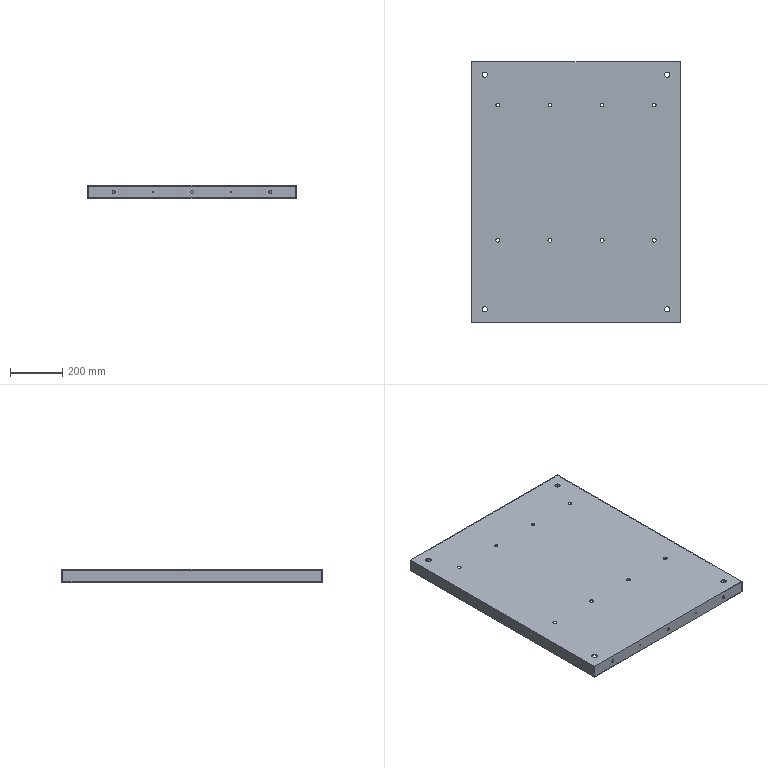Part | SolidWorks | features BaseBody 1 | 1 solid | 89 faces | box 800 x 1000 x 50 mm | volume 2747861 mm3 | cylinder 60 | plane 29 | commonest cylinder face diameters 10.6 x26 20 x14 14 x8 15 x8 4.4 x4